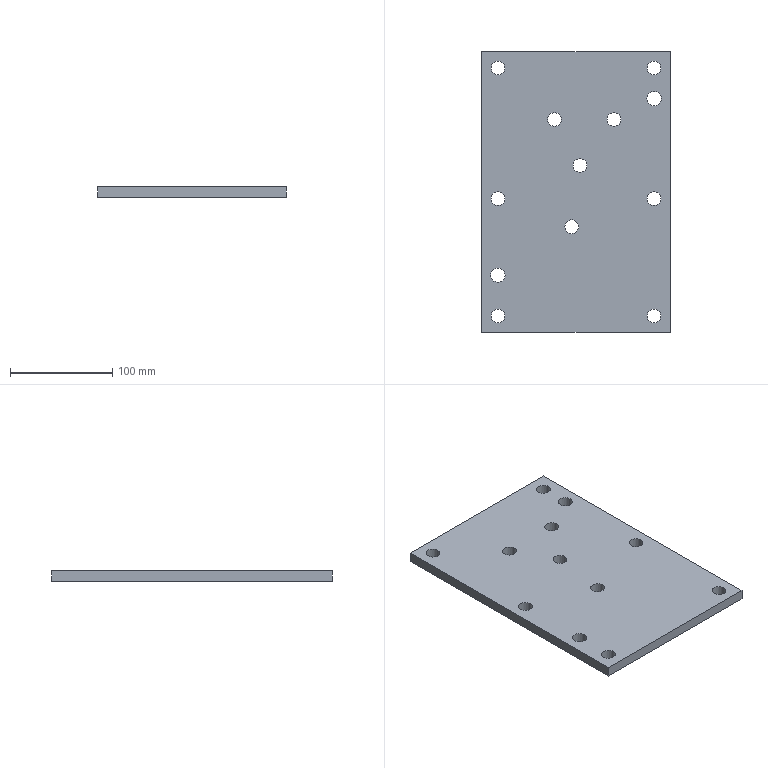Part | STEP file | lll_id2966_x_t | 1 solid | 18 faces | box 185 x 275 x 10 mm | volume 491338 mm3 | cylinder 12 | plane 6 | commonest cylinder face diameters 13.509 x10 14 x2
STEP:
#1=CARTESIAN_POINT('',(1348.816,217.359,92.5));
#2=VERTEX_POINT('',#1);
#3=CARTESIAN_POINT('',(1342.062,217.359,92.5));
#4=DIRECTION('',(0.,0.,1.));
#5=DIRECTION('',(1.,0.,0.));
#6=AXIS2_PLACEMENT_3D('',#3,#4,#5);
#7=CIRCLE('',#6,6.755);
#8=EDGE_CURVE('',#2,#2,#7,.T.);
#9=ORIENTED_EDGE('',*,*,#8,.T.);
#10=EDGE_LOOP('',(#9));
#11=FACE_BOUND('',#10,.T.);
#12=CARTESIAN_POINT('',(1390.082,322.359,92.5));
#13=VERTEX_POINT('',#12);
#14=CARTESIAN_POINT('',(1383.328,322.359,92.5));
#15=DIRECTION('',(0.,0.,1.));
#16=DIRECTION('',(1.,0.,0.));
#17=AXIS2_PLACEMENT_3D('',#14,#15,#16);
#18=CIRCLE('',#17,6.755);
#19=EDGE_CURVE('',#13,#13,#18,.T.);
#20=ORIENTED_EDGE('',*,*,#19,.T.);
#21=EDGE_LOOP('',(#20));
#22=FACE_BOUND('',#21,.T.);
#23=CARTESIAN_POINT('',(1415.917,244.859,92.5));
#24=VERTEX_POINT('',#23);
#25=CARTESIAN_POINT('',(1422.671,244.859,92.5));
#26=DIRECTION('',(0.,0.,-1.));
#27=DIRECTION('',(-1.,0.,0.));
#28=AXIS2_PLACEMENT_3D('',#25,#26,#27);
#29=CIRCLE('',#28,6.755);
#30=EDGE_CURVE('',#24,#24,#29,.T.);
#31=ORIENTED_EDGE('',*,*,#30,.F.);
#32=EDGE_LOOP('',(#31));
#33=FACE_BOUND('',#32,.T.);
#34=CARTESIAN_POINT('',(1262.917,244.859,92.5));
#35=VERTEX_POINT('',#34);
#36=CARTESIAN_POINT('',(1269.671,244.859,92.5));
#37=DIRECTION('',(0.,0.,-1.));
#38=DIRECTION('',(-1.,0.,0.));
#39=AXIS2_PLACEMENT_3D('',#36,#37,#38);
#40=CIRCLE('',#39,6.755);
#41=EDGE_CURVE('',#35,#35,#40,.T.);
#42=ORIENTED_EDGE('',*,*,#41,.F.);
#43=EDGE_LOOP('',(#42));
#44=FACE_BOUND('',#43,.T.);
#45=CARTESIAN_POINT('',(1262.671,169.859,92.5));
#46=VERTEX_POINT('',#45);
#47=CARTESIAN_POINT('',(1269.671,169.859,92.5));
#48=DIRECTION('',(0.,0.,1.));
#49=DIRECTION('',(-1.,0.,0.));
#50=AXIS2_PLACEMENT_3D('',#47,#48,#49);
#51=CIRCLE('',#50,7.);
#52=EDGE_CURVE('',#46,#46,#51,.T.);
#53=ORIENTED_EDGE('',*,*,#52,.T.);
#54=EDGE_LOOP('',(#53));
#55=FACE_BOUND('',#54,.T.);
#56=CARTESIAN_POINT('',(1415.917,129.859,92.5));
#57=VERTEX_POINT('',#56);
#58=CARTESIAN_POINT('',(1422.671,129.859,92.5));
#59=DIRECTION('',(0.,0.,1.));
#60=DIRECTION('',(-1.,0.,0.));
#61=AXIS2_PLACEMENT_3D('',#58,#59,#60);
#62=CIRCLE('',#61,6.755);
#63=EDGE_CURVE('',#57,#57,#62,.T.);
#64=ORIENTED_EDGE('',*,*,#63,.T.);
#65=EDGE_LOOP('',(#64));
#66=FACE_BOUND('',#65,.T.);
#67=CARTESIAN_POINT('',(1262.917,129.859,92.5));
#68=VERTEX_POINT('',#67);
#69=CARTESIAN_POINT('',(1269.671,129.859,92.5));
#70=DIRECTION('',(0.,0.,1.));
#71=DIRECTION('',(-1.,0.,0.));
#72=AXIS2_PLACEMENT_3D('',#69,#70,#71);
#73=CIRCLE('',#72,6.755);
#74=EDGE_CURVE('',#68,#68,#73,.T.);
#75=ORIENTED_EDGE('',*,*,#74,.T.);
#76=EDGE_LOOP('',(#75));
#77=FACE_BOUND('',#76,.T.);
#78=CARTESIAN_POINT('',(1253.671,388.859,92.5));
#79=VERTEX_POINT('',#78);
#80=CARTESIAN_POINT('',(1253.671,113.859,92.5));
#81=VERTEX_POINT('',#80);
#82=CARTESIAN_POINT('',(1253.671,251.359,92.5));
#83=DIRECTION('',(0.,-1.,0.));
#84=VECTOR('',#83,1.);
#85=LINE('',#82,#84);
#86=EDGE_CURVE('',#79,#81,#85,.T.);
#87=ORIENTED_EDGE('',*,*,#86,.F.);
#88=CARTESIAN_POINT('',(1438.671,388.859,92.5));
#89=VERTEX_POINT('',#88);
#90=CARTESIAN_POINT('',(1346.171,388.859,92.5));
#91=DIRECTION('',(-1.,0.,0.));
#92=VECTOR('',#91,1.);
#93=LINE('',#90,#92);
#94=EDGE_CURVE('',#89,#79,#93,.T.);
#95=ORIENTED_EDGE('',*,*,#94,.F.);
#96=CARTESIAN_POINT('',(1438.671,113.859,92.5));
#97=VERTEX_POINT('',#96);
#98=CARTESIAN_POINT('',(1438.671,251.359,92.5));
#99=DIRECTION('',(0.,1.,0.));
#100=VECTOR('',#99,1.);
#101=LINE('',#98,#100);
#102=EDGE_CURVE('',#97,#89,#101,.T.);
#103=ORIENTED_EDGE('',*,*,#102,.F.);
#104=CARTESIAN_POINT('',(1346.171,113.859,92.5));
#105=DIRECTION('',(1.,0.,0.));
#106=VECTOR('',#105,1.);
#107=LINE('',#104,#106);
#108=EDGE_CURVE('',#81,#97,#107,.T.);
#109=ORIENTED_EDGE('',*,*,#108,.F.);
#110=EDGE_LOOP('',(#87,#95,#103,#109));
#111=FACE_BOUND('',#110,.T.);
#112=CARTESIAN_POINT('',(1415.917,372.859,92.5));
#113=VERTEX_POINT('',#112);
#114=CARTESIAN_POINT('',(1422.671,372.859,92.5));
#115=DIRECTION('',(0.,0.,1.));
#116=DIRECTION('',(-1.,0.,0.));
#117=AXIS2_PLACEMENT_3D('',#114,#115,#116);
#118=CIRCLE('',#117,6.755);
#119=EDGE_CURVE('',#113,#113,#118,.T.);
#120=ORIENTED_EDGE('',*,*,#119,.T.);
#121=EDGE_LOOP('',(#120));
#122=FACE_BOUND('',#121,.T.);
#123=CARTESIAN_POINT('',(1262.917,372.859,92.5));
#124=VERTEX_POINT('',#123);
#125=CARTESIAN_POINT('',(1269.671,372.859,92.5));
#126=DIRECTION('',(0.,0.,1.));
#127=DIRECTION('',(-1.,0.,0.));
#128=AXIS2_PLACEMENT_3D('',#125,#126,#127);
#129=CIRCLE('',#128,6.755);
#130=EDGE_CURVE('',#124,#124,#129,.T.);
#131=ORIENTED_EDGE('',*,*,#130,.T.);
#132=EDGE_LOOP('',(#131));
#133=FACE_BOUND('',#132,.T.);
#134=CARTESIAN_POINT('',(1415.671,342.859,92.5));
#135=VERTEX_POINT('',#134);
#136=CARTESIAN_POINT('',(1422.671,342.859,92.5));
#137=DIRECTION('',(0.,0.,1.));
#138=DIRECTION('',(-1.,0.,0.));
#139=AXIS2_PLACEMENT_3D('',#136,#137,#138);
#140=CIRCLE('',#139,7.);
#141=EDGE_CURVE('',#135,#135,#140,.T.);
#142=ORIENTED_EDGE('',*,*,#141,.T.);
#143=EDGE_LOOP('',(#142));
#144=FACE_BOUND('',#143,.T.);
#145=CARTESIAN_POINT('',(1356.816,277.359,92.5));
#146=VERTEX_POINT('',#145);
#147=CARTESIAN_POINT('',(1350.062,277.359,92.5));
#148=DIRECTION('',(0.,0.,1.));
#149=DIRECTION('',(1.,0.,0.));
#150=AXIS2_PLACEMENT_3D('',#147,#148,#149);
#151=CIRCLE('',#150,6.755);
#152=EDGE_CURVE('',#146,#146,#151,.T.);
#153=ORIENTED_EDGE('',*,*,#152,.T.);
#154=EDGE_LOOP('',(#153));
#155=FACE_BOUND('',#154,.T.);
#156=CARTESIAN_POINT('',(1331.816,322.359,92.5));
#157=VERTEX_POINT('',#156);
#158=CARTESIAN_POINT('',(1325.062,322.359,92.5));
#159=DIRECTION('',(0.,0.,1.));
#160=DIRECTION('',(1.,0.,0.));
#161=AXIS2_PLACEMENT_3D('',#158,#159,#160);
#162=CIRCLE('',#161,6.755);
#163=EDGE_CURVE('',#157,#157,#162,.T.);
#164=ORIENTED_EDGE('',*,*,#163,.T.);
#165=EDGE_LOOP('',(#164));
#166=FACE_BOUND('',#165,.T.);
#167=CARTESIAN_POINT('',(1346.171,251.359,92.5));
#168=DIRECTION('',(0.,0.,-1.));
#169=DIRECTION('',(1.,0.,0.));
#170=AXIS2_PLACEMENT_3D('',#167,#168,#169);
#171=PLANE('',#170);
#172=ADVANCED_FACE('',(#11,#22,#33,#44,#55,#66,#77,#111,#122,#133,#144,#155,#166),#171,.T.);
#173=CARTESIAN_POINT('',(1335.307,217.359,102.5));
#174=VERTEX_POINT('',#173);
#175=CARTESIAN_POINT('',(1342.062,217.359,102.5));
#176=DIRECTION('',(0.,0.,1.));
#177=DIRECTION('',(-1.,0.,0.));
#178=AXIS2_PLACEMENT_3D('',#175,#176,#177);
#179=CIRCLE('',#178,6.755);
#180=EDGE_CURVE('',#174,#174,#179,.T.);
#181=ORIENTED_EDGE('',*,*,#180,.F.);
#182=EDGE_LOOP('',(#181));
#183=FACE_BOUND('',#182,.T.);
#184=CARTESIAN_POINT('',(1376.573,322.359,102.5));
#185=VERTEX_POINT('',#184);
#186=CARTESIAN_POINT('',(1383.328,322.359,102.5));
#187=DIRECTION('',(0.,0.,1.));
#188=DIRECTION('',(-1.,0.,0.));
#189=AXIS2_PLACEMENT_3D('',#186,#187,#188);
#190=CIRCLE('',#189,6.755);
#191=EDGE_CURVE('',#185,#185,#190,.T.);
#192=ORIENTED_EDGE('',*,*,#191,.F.);
#193=EDGE_LOOP('',(#192));
#194=FACE_BOUND('',#193,.T.);
#195=CARTESIAN_POINT('',(1415.671,342.859,102.5));
#196=VERTEX_POINT('',#195);
#197=CARTESIAN_POINT('',(1422.671,342.859,102.5));
#198=DIRECTION('',(0.,0.,-1.));
#199=DIRECTION('',(-1.,0.,0.));
#200=AXIS2_PLACEMENT_3D('',#197,#198,#199);
#201=CIRCLE('',#200,7.);
#202=EDGE_CURVE('',#196,#196,#201,.T.);
#203=ORIENTED_EDGE('',*,*,#202,.T.);
#204=EDGE_LOOP('',(#203));
#205=FACE_BOUND('',#204,.T.);
#206=CARTESIAN_POINT('',(1415.917,372.859,102.5));
#207=VERTEX_POINT('',#206);
#208=CARTESIAN_POINT('',(1422.671,372.859,102.5));
#209=DIRECTION('',(0.,0.,-1.));
#210=DIRECTION('',(-1.,0.,0.));
#211=AXIS2_PLACEMENT_3D('',#208,#209,#210);
#212=CIRCLE('',#211,6.755);
#213=EDGE_CURVE('',#207,#207,#212,.T.);
#214=ORIENTED_EDGE('',*,*,#213,.T.);
#215=EDGE_LOOP('',(#214));
#216=FACE_BOUND('',#215,.T.);
#217=CARTESIAN_POINT('',(1438.671,388.859,102.5));
#218=VERTEX_POINT('',#217);
#219=CARTESIAN_POINT('',(1438.671,113.859,102.5));
#220=VERTEX_POINT('',#219);
#221=CARTESIAN_POINT('',(1438.671,251.359,102.5));
#222=DIRECTION('',(0.,-1.,0.));
#223=VECTOR('',#222,1.);
#224=LINE('',#221,#223);
#225=EDGE_CURVE('',#218,#220,#224,.T.);
#226=ORIENTED_EDGE('',*,*,#225,.F.);
#227=CARTESIAN_POINT('',(1253.671,388.859,102.5));
#228=VERTEX_POINT('',#227);
#229=CARTESIAN_POINT('',(1346.171,388.859,102.5));
#230=DIRECTION('',(-1.,0.,0.));
#231=VECTOR('',#230,1.);
#232=LINE('',#229,#231);
#233=EDGE_CURVE('',#218,#228,#232,.T.);
#234=ORIENTED_EDGE('',*,*,#233,.T.);
#235=CARTESIAN_POINT('',(1253.671,113.859,102.5));
#236=VERTEX_POINT('',#235);
#237=CARTESIAN_POINT('',(1253.671,251.359,102.5));
#238=DIRECTION('',(0.,1.,0.));
#239=VECTOR('',#238,1.);
#240=LINE('',#237,#239);
#241=EDGE_CURVE('',#236,#228,#240,.T.);
#242=ORIENTED_EDGE('',*,*,#241,.F.);
#243=CARTESIAN_POINT('',(1346.171,113.859,102.5));
#244=DIRECTION('',(-1.,0.,0.));
#245=VECTOR('',#244,1.);
#246=LINE('',#243,#245);
#247=EDGE_CURVE('',#220,#236,#246,.T.);
#248=ORIENTED_EDGE('',*,*,#247,.F.);
#249=EDGE_LOOP('',(#226,#234,#242,#248));
#250=FACE_BOUND('',#249,.T.);
#251=CARTESIAN_POINT('',(1415.917,129.859,102.5));
#252=VERTEX_POINT('',#251);
#253=CARTESIAN_POINT('',(1422.671,129.859,102.5));
#254=DIRECTION('',(0.,0.,1.));
#255=DIRECTION('',(-1.,0.,0.));
#256=AXIS2_PLACEMENT_3D('',#253,#254,#255);
#257=CIRCLE('',#256,6.755);
#258=EDGE_CURVE('',#252,#252,#257,.T.);
#259=ORIENTED_EDGE('',*,*,#258,.F.);
#260=EDGE_LOOP('',(#259));
#261=FACE_BOUND('',#260,.T.);
#262=CARTESIAN_POINT('',(1415.917,244.859,102.5));
#263=VERTEX_POINT('',#262);
#264=CARTESIAN_POINT('',(1422.671,244.859,102.5));
#265=DIRECTION('',(0.,0.,-1.));
#266=DIRECTION('',(-1.,0.,0.));
#267=AXIS2_PLACEMENT_3D('',#264,#265,#266);
#268=CIRCLE('',#267,6.755);
#269=EDGE_CURVE('',#263,#263,#268,.T.);
#270=ORIENTED_EDGE('',*,*,#269,.T.);
#271=EDGE_LOOP('',(#270));
#272=FACE_BOUND('',#271,.T.);
#273=CARTESIAN_POINT('',(1262.917,244.859,102.5));
#274=VERTEX_POINT('',#273);
#275=CARTESIAN_POINT('',(1269.671,244.859,102.5));
#276=DIRECTION('',(0.,0.,-1.));
#277=DIRECTION('',(-1.,0.,0.));
#278=AXIS2_PLACEMENT_3D('',#275,#276,#277);
#279=CIRCLE('',#278,6.755);
#280=EDGE_CURVE('',#274,#274,#279,.T.);
#281=ORIENTED_EDGE('',*,*,#280,.T.);
#282=EDGE_LOOP('',(#281));
#283=FACE_BOUND('',#282,.T.);
#284=CARTESIAN_POINT('',(1262.671,169.859,102.5));
#285=VERTEX_POINT('',#284);
#286=CARTESIAN_POINT('',(1269.671,169.859,102.5));
#287=DIRECTION('',(0.,0.,1.));
#288=DIRECTION('',(-1.,0.,0.));
#289=AXIS2_PLACEMENT_3D('',#286,#287,#288);
#290=CIRCLE('',#289,7.);
#291=EDGE_CURVE('',#285,#285,#290,.T.);
#292=ORIENTED_EDGE('',*,*,#291,.F.);
#293=EDGE_LOOP('',(#292));
#294=FACE_BOUND('',#293,.T.);
#295=CARTESIAN_POINT('',(1262.917,129.859,102.5));
#296=VERTEX_POINT('',#295);
#297=CARTESIAN_POINT('',(1269.671,129.859,102.5));
#298=DIRECTION('',(0.,0.,-1.));
#299=DIRECTION('',(-1.,0.,0.));
#300=AXIS2_PLACEMENT_3D('',#297,#298,#299);
#301=CIRCLE('',#300,6.755);
#302=EDGE_CURVE('',#296,#296,#301,.T.);
#303=ORIENTED_EDGE('',*,*,#302,.T.);
#304=EDGE_LOOP('',(#303));
#305=FACE_BOUND('',#304,.T.);
#306=CARTESIAN_POINT('',(1262.917,372.859,102.5));
#307=VERTEX_POINT('',#306);
#308=CARTESIAN_POINT('',(1269.671,372.859,102.5));
#309=DIRECTION('',(0.,0.,-1.));
#310=DIRECTION('',(-1.,0.,0.));
#311=AXIS2_PLACEMENT_3D('',#308,#309,#310);
#312=CIRCLE('',#311,6.755);
#313=EDGE_CURVE('',#307,#307,#312,.T.);
#314=ORIENTED_EDGE('',*,*,#313,.T.);
#315=EDGE_LOOP('',(#314));
#316=FACE_BOUND('',#315,.T.);
#317=CARTESIAN_POINT('',(1343.307,277.359,102.5));
#318=VERTEX_POINT('',#317);
#319=CARTESIAN_POINT('',(1350.062,277.359,102.5));
#320=DIRECTION('',(0.,0.,1.));
#321=DIRECTION('',(-1.,0.,0.));
#322=AXIS2_PLACEMENT_3D('',#319,#320,#321);
#323=CIRCLE('',#322,6.755);
#324=EDGE_CURVE('',#318,#318,#323,.T.);
#325=ORIENTED_EDGE('',*,*,#324,.F.);
#326=EDGE_LOOP('',(#325));
#327=FACE_BOUND('',#326,.T.);
#328=CARTESIAN_POINT('',(1318.307,322.359,102.5));
#329=VERTEX_POINT('',#328);
#330=CARTESIAN_POINT('',(1325.062,322.359,102.5));
#331=DIRECTION('',(0.,0.,1.));
#332=DIRECTION('',(-1.,0.,0.));
#333=AXIS2_PLACEMENT_3D('',#330,#331,#332);
#334=CIRCLE('',#333,6.755);
#335=EDGE_CURVE('',#329,#329,#334,.T.);
#336=ORIENTED_EDGE('',*,*,#335,.F.);
#337=EDGE_LOOP('',(#336));
#338=FACE_BOUND('',#337,.T.);
#339=CARTESIAN_POINT('',(1346.171,251.359,102.5));
#340=DIRECTION('',(0.,0.,-1.));
#341=DIRECTION('',(-1.,0.,0.));
#342=AXIS2_PLACEMENT_3D('',#339,#340,#341);
#343=PLANE('',#342);
#344=ADVANCED_FACE('',(#183,#194,#205,#216,#250,#261,#272,#283,#294,#305,#316,#327,#338),#343,.F.);
#345=ORIENTED_EDGE('',*,*,#202,.F.);
#346=EDGE_LOOP('',(#345));
#347=FACE_BOUND('',#346,.T.);
#348=ORIENTED_EDGE('',*,*,#141,.F.);
#349=EDGE_LOOP('',(#348));
#350=FACE_BOUND('',#349,.T.);
#351=CARTESIAN_POINT('',(1422.671,342.859,92.5));
#352=DIRECTION('',(0.,0.,1.));
#353=DIRECTION('',(-1.,0.,0.));
#354=AXIS2_PLACEMENT_3D('',#351,#352,#353);
#355=CYLINDRICAL_SURFACE('',#354,7.);
#356=ADVANCED_FACE('',(#347,#350),#355,.F.);
#357=ORIENTED_EDGE('',*,*,#313,.F.);
#358=EDGE_LOOP('',(#357));
#359=FACE_BOUND('',#358,.T.);
#360=ORIENTED_EDGE('',*,*,#130,.F.);
#361=EDGE_LOOP('',(#360));
#362=FACE_BOUND('',#361,.T.);
#363=CARTESIAN_POINT('',(1269.671,372.859,92.5));
#364=DIRECTION('',(0.,0.,1.));
#365=DIRECTION('',(-1.,0.,0.));
#366=AXIS2_PLACEMENT_3D('',#363,#364,#365);
#367=CYLINDRICAL_SURFACE('',#366,6.755);
#368=ADVANCED_FACE('',(#359,#362),#367,.F.);
#369=ORIENTED_EDGE('',*,*,#213,.F.);
#370=EDGE_LOOP('',(#369));
#371=FACE_BOUND('',#370,.T.);
#372=ORIENTED_EDGE('',*,*,#119,.F.);
#373=EDGE_LOOP('',(#372));
#374=FACE_BOUND('',#373,.T.);
#375=CARTESIAN_POINT('',(1422.671,372.859,92.5));
#376=DIRECTION('',(0.,0.,1.));
#377=DIRECTION('',(-1.,0.,0.));
#378=AXIS2_PLACEMENT_3D('',#375,#376,#377);
#379=CYLINDRICAL_SURFACE('',#378,6.755);
#380=ADVANCED_FACE('',(#371,#374),#379,.F.);
#381=ORIENTED_EDGE('',*,*,#233,.F.);
#382=CARTESIAN_POINT('',(1438.671,388.859,92.5));
#383=DIRECTION('',(0.,0.,1.));
#384=VECTOR('',#383,1.);
#385=LINE('',#382,#384);
#386=EDGE_CURVE('',#89,#218,#385,.T.);
#387=ORIENTED_EDGE('',*,*,#386,.F.);
#388=ORIENTED_EDGE('',*,*,#94,.T.);
#389=CARTESIAN_POINT('',(1253.671,388.859,92.5));
#390=DIRECTION('',(0.,0.,1.));
#391=VECTOR('',#390,1.);
#392=LINE('',#389,#391);
#393=EDGE_CURVE('',#79,#228,#392,.T.);
#394=ORIENTED_EDGE('',*,*,#393,.T.);
#395=EDGE_LOOP('',(#381,#387,#388,#394));
#396=FACE_OUTER_BOUND('',#395,.T.);
#397=CARTESIAN_POINT('',(1346.171,388.859,92.5));
#398=DIRECTION('',(0.,1.,0.));
#399=DIRECTION('',(0.,0.,-1.));
#400=AXIS2_PLACEMENT_3D('',#397,#398,#399);
#401=PLANE('',#400);
#402=ADVANCED_FACE('',(#396),#401,.T.);
#403=ORIENTED_EDGE('',*,*,#241,.T.);
#404=ORIENTED_EDGE('',*,*,#393,.F.);
#405=ORIENTED_EDGE('',*,*,#86,.T.);
#406=CARTESIAN_POINT('',(1253.671,113.859,92.5));
#407=DIRECTION('',(0.,0.,1.));
#408=VECTOR('',#407,1.);
#409=LINE('',#406,#408);
#410=EDGE_CURVE('',#81,#236,#409,.T.);
#411=ORIENTED_EDGE('',*,*,#410,.T.);
#412=EDGE_LOOP('',(#403,#404,#405,#411));
#413=FACE_OUTER_BOUND('',#412,.T.);
#414=CARTESIAN_POINT('',(1253.671,251.359,92.5));
#415=DIRECTION('',(-1.,0.,0.));
#416=DIRECTION('',(0.,0.,-1.));
#417=AXIS2_PLACEMENT_3D('',#414,#415,#416);
#418=PLANE('',#417);
#419=ADVANCED_FACE('',(#413),#418,.T.);
#420=ORIENTED_EDGE('',*,*,#247,.T.);
#421=ORIENTED_EDGE('',*,*,#410,.F.);
#422=ORIENTED_EDGE('',*,*,#108,.T.);
#423=CARTESIAN_POINT('',(1438.671,113.859,92.5));
#424=DIRECTION('',(0.,0.,1.));
#425=VECTOR('',#424,1.);
#426=LINE('',#423,#425);
#427=EDGE_CURVE('',#97,#220,#426,.T.);
#428=ORIENTED_EDGE('',*,*,#427,.T.);
#429=EDGE_LOOP('',(#420,#421,#422,#428));
#430=FACE_OUTER_BOUND('',#429,.T.);
#431=CARTESIAN_POINT('',(1346.171,113.859,92.5));
#432=DIRECTION('',(0.,-1.,0.));
#433=DIRECTION('',(0.,0.,1.));
#434=AXIS2_PLACEMENT_3D('',#431,#432,#433);
#435=PLANE('',#434);
#436=ADVANCED_FACE('',(#430),#435,.T.);
#437=ORIENTED_EDGE('',*,*,#225,.T.);
#438=ORIENTED_EDGE('',*,*,#427,.F.);
#439=ORIENTED_EDGE('',*,*,#102,.T.);
#440=ORIENTED_EDGE('',*,*,#386,.T.);
#441=EDGE_LOOP('',(#437,#438,#439,#440));
#442=FACE_OUTER_BOUND('',#441,.T.);
#443=CARTESIAN_POINT('',(1438.671,251.359,92.5));
#444=DIRECTION('',(1.,0.,0.));
#445=DIRECTION('',(0.,0.,1.));
#446=AXIS2_PLACEMENT_3D('',#443,#444,#445);
#447=PLANE('',#446);
#448=ADVANCED_FACE('',(#442),#447,.T.);
#449=ORIENTED_EDGE('',*,*,#302,.F.);
#450=EDGE_LOOP('',(#449));
#451=FACE_BOUND('',#450,.T.);
#452=ORIENTED_EDGE('',*,*,#74,.F.);
#453=EDGE_LOOP('',(#452));
#454=FACE_BOUND('',#453,.T.);
#455=CARTESIAN_POINT('',(1269.671,129.859,92.5));
#456=DIRECTION('',(0.,0.,1.));
#457=DIRECTION('',(-1.,0.,0.));
#458=AXIS2_PLACEMENT_3D('',#455,#456,#457);
#459=CYLINDRICAL_SURFACE('',#458,6.755);
#460=ADVANCED_FACE('',(#451,#454),#459,.F.);
#461=ORIENTED_EDGE('',*,*,#258,.T.);
#462=EDGE_LOOP('',(#461));
#463=FACE_BOUND('',#462,.T.);
#464=ORIENTED_EDGE('',*,*,#63,.F.);
#465=EDGE_LOOP('',(#464));
#466=FACE_BOUND('',#465,.T.);
#467=CARTESIAN_POINT('',(1422.671,129.859,92.5));
#468=DIRECTION('',(0.,0.,1.));
#469=DIRECTION('',(-1.,0.,0.));
#470=AXIS2_PLACEMENT_3D('',#467,#468,#469);
#471=CYLINDRICAL_SURFACE('',#470,6.755);
#472=ADVANCED_FACE('',(#463,#466),#471,.F.);
#473=ORIENTED_EDGE('',*,*,#291,.T.);
#474=EDGE_LOOP('',(#473));
#475=FACE_BOUND('',#474,.T.);
#476=ORIENTED_EDGE('',*,*,#52,.F.);
#477=EDGE_LOOP('',(#476));
#478=FACE_BOUND('',#477,.T.);
#479=CARTESIAN_POINT('',(1269.671,169.859,92.5));
#480=DIRECTION('',(0.,0.,1.));
#481=DIRECTION('',(-1.,0.,0.));
#482=AXIS2_PLACEMENT_3D('',#479,#480,#481);
#483=CYLINDRICAL_SURFACE('',#482,7.);
#484=ADVANCED_FACE('',(#475,#478),#483,.F.);
#485=ORIENTED_EDGE('',*,*,#280,.F.);
#486=EDGE_LOOP('',(#485));
#487=FACE_BOUND('',#486,.T.);
#488=ORIENTED_EDGE('',*,*,#41,.T.);
#489=EDGE_LOOP('',(#488));
#490=FACE_BOUND('',#489,.T.);
#491=CARTESIAN_POINT('',(1269.671,244.859,92.5));
#492=DIRECTION('',(0.,0.,1.));
#493=DIRECTION('',(-1.,0.,0.));
#494=AXIS2_PLACEMENT_3D('',#491,#492,#493);
#495=CYLINDRICAL_SURFACE('',#494,6.755);
#496=ADVANCED_FACE('',(#487,#490),#495,.F.);
#497=ORIENTED_EDGE('',*,*,#269,.F.);
#498=EDGE_LOOP('',(#497));
#499=FACE_BOUND('',#498,.T.);
#500=ORIENTED_EDGE('',*,*,#30,.T.);
#501=EDGE_LOOP('',(#500));
#502=FACE_BOUND('',#501,.T.);
#503=CARTESIAN_POINT('',(1422.671,244.859,92.5));
#504=DIRECTION('',(0.,0.,1.));
#505=DIRECTION('',(-1.,0.,0.));
#506=AXIS2_PLACEMENT_3D('',#503,#504,#505);
#507=CYLINDRICAL_SURFACE('',#506,6.755);
#508=ADVANCED_FACE('',(#499,#502),#507,.F.);
#509=ORIENTED_EDGE('',*,*,#19,.F.);
#510=EDGE_LOOP('',(#509));
#511=FACE_BOUND('',#510,.T.);
#512=ORIENTED_EDGE('',*,*,#191,.T.);
#513=EDGE_LOOP('',(#512));
#514=FACE_BOUND('',#513,.T.);
#515=CARTESIAN_POINT('',(1383.328,322.359,337.5));
#516=DIRECTION('',(0.,0.,-1.));
#517=DIRECTION('',(-1.,0.,0.));
#518=AXIS2_PLACEMENT_3D('',#515,#516,#517);
#519=CYLINDRICAL_SURFACE('',#518,6.755);
#520=ADVANCED_FACE('',(#511,#514),#519,.F.);
#521=ORIENTED_EDGE('',*,*,#152,.F.);
#522=EDGE_LOOP('',(#521));
#523=FACE_BOUND('',#522,.T.);
#524=ORIENTED_EDGE('',*,*,#324,.T.);
#525=EDGE_LOOP('',(#524));
#526=FACE_BOUND('',#525,.T.);
#527=CARTESIAN_POINT('',(1350.062,277.359,337.5));
#528=DIRECTION('',(0.,0.,-1.));
#529=DIRECTION('',(-1.,0.,0.));
#530=AXIS2_PLACEMENT_3D('',#527,#528,#529);
#531=CYLINDRICAL_SURFACE('',#530,6.755);
#532=ADVANCED_FACE('',(#523,#526),#531,.F.);
#533=ORIENTED_EDGE('',*,*,#8,.F.);
#534=EDGE_LOOP('',(#533));
#535=FACE_BOUND('',#534,.T.);
#536=ORIENTED_EDGE('',*,*,#180,.T.);
#537=EDGE_LOOP('',(#536));
#538=FACE_BOUND('',#537,.T.);
#539=CARTESIAN_POINT('',(1342.062,217.359,337.5));
#540=DIRECTION('',(0.,0.,-1.));
#541=DIRECTION('',(-1.,0.,0.));
#542=AXIS2_PLACEMENT_3D('',#539,#540,#541);
#543=CYLINDRICAL_SURFACE('',#542,6.755);
#544=ADVANCED_FACE('',(#535,#538),#543,.F.);
#545=ORIENTED_EDGE('',*,*,#163,.F.);
#546=EDGE_LOOP('',(#545));
#547=FACE_BOUND('',#546,.T.);
#548=ORIENTED_EDGE('',*,*,#335,.T.);
#549=EDGE_LOOP('',(#548));
#550=FACE_BOUND('',#549,.T.);
#551=CARTESIAN_POINT('',(1325.062,322.359,337.5));
#552=DIRECTION('',(0.,0.,-1.));
#553=DIRECTION('',(-1.,0.,0.));
#554=AXIS2_PLACEMENT_3D('',#551,#552,#553);
#555=CYLINDRICAL_SURFACE('',#554,6.755);
#556=ADVANCED_FACE('',(#547,#550),#555,.F.);
#557=CLOSED_SHELL('',(#172,#344,#356,#368,#380,#402,#419,#436,#448,#460,#472,#484,#496,#508,#520,#532,#544,#556));
#558=MANIFOLD_SOLID_BREP('',#557);
#559=(LENGTH_UNIT()NAMED_UNIT(*)SI_UNIT(.MILLI.,.METRE.));
#560=UNCERTAINTY_MEASURE_WITH_UNIT(LENGTH_MEASURE(0.00002),#559,'','');
#561=(NAMED_UNIT(*)PLANE_ANGLE_UNIT()SI_UNIT($,.RADIAN.));
#562=PLANE_ANGLE_MEASURE_WITH_UNIT(PLANE_ANGLE_MEASURE(0.01745),#561);
#563=DIMENSIONAL_EXPONENTS(0.,0.,0.,0.,0.,0.,0.);
#564=(CONVERSION_BASED_UNIT('DEGREE',#562)NAMED_UNIT(#563)PLANE_ANGLE_UNIT());
#565=(NAMED_UNIT(*)SI_UNIT($,.STERADIAN.)SOLID_ANGLE_UNIT());
#566=(GEOMETRIC_REPRESENTATION_CONTEXT(3)GLOBAL_UNCERTAINTY_ASSIGNED_CONTEXT((#560))GLOBAL_UNIT_ASSIGNED_CONTEXT((#559,#564,#565))REPRESENTATION_CONTEXT('',''));
#567=ADVANCED_BREP_SHAPE_REPRESENTATION('',(#558),#566);